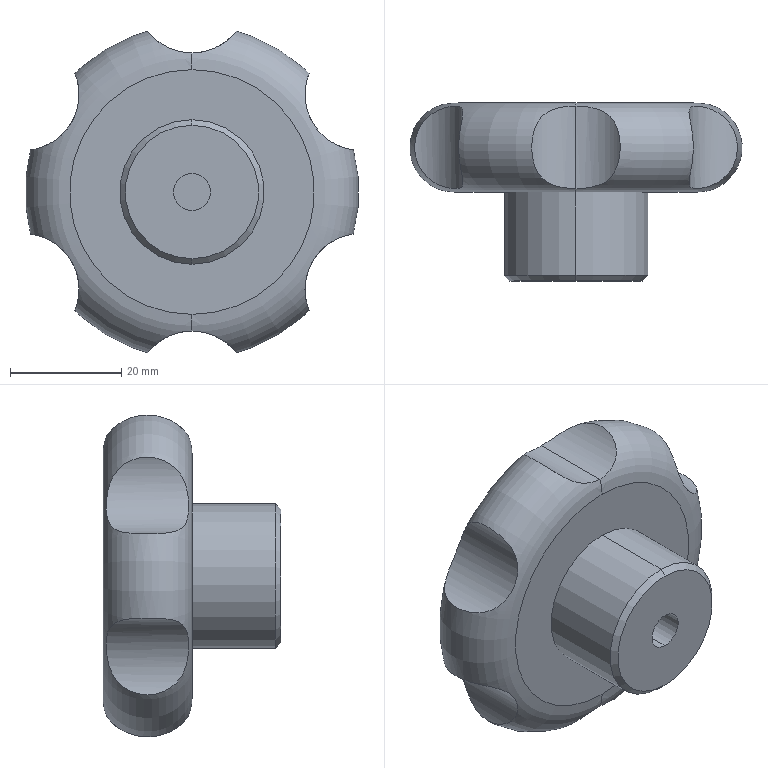Part | STEP file | 001-003-HAK13-D60-M8 | 1 solid | 22 faces | box 60 x 32 x 57.857 mm | volume 42793 mm3 | cylinder 11 | plane 5 | cone 4 | torus 2 | commonest cylinder face diameters 20 x7 6.647 x2 26 x2